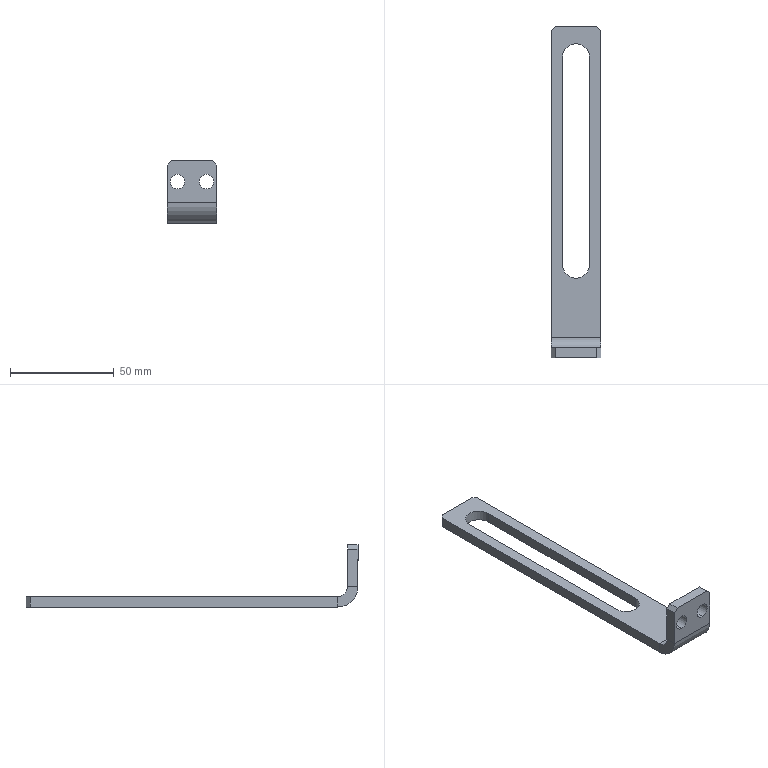Part | SolidWorks | 1 solid | 26 faces | box 24 x 160 x 30 mm | volume 14225 mm3 | plane 18 | cylinder 8 | commonest cylinder face diameters 7 x4 13 x2 10 x1 20 x1
STEP:
#1=CARTESIAN_POINT('',(-7.,-80.,18.5));
#2=VERTEX_POINT('',#1);
#3=CARTESIAN_POINT('',(-7.,-80.,11.5));
#4=VERTEX_POINT('',#3);
#5=CARTESIAN_POINT('',(-7.,-80.,15.));
#6=DIRECTION('',(0.,-1.,0.));
#7=DIRECTION('',(0.,0.,-1.));
#8=AXIS2_PLACEMENT_3D('',#5,#6,#7);
#9=CIRCLE('',#8,3.5);
#10=EDGE_CURVE('',#2,#4,#9,.T.);
#11=ORIENTED_EDGE('',*,*,#10,.T.);
#12=CARTESIAN_POINT('',(-7.,-75.,11.5));
#13=VERTEX_POINT('',#12);
#14=CARTESIAN_POINT('',(-7.,-85.,11.5));
#15=DIRECTION('',(0.,1.,0.));
#16=VECTOR('',#15,1000.);
#17=LINE('',#14,#16);
#18=EDGE_CURVE('',#4,#13,#17,.T.);
#19=ORIENTED_EDGE('',*,*,#18,.T.);
#20=CARTESIAN_POINT('',(-7.,-75.,18.5));
#21=VERTEX_POINT('',#20);
#22=CARTESIAN_POINT('',(-7.,-75.,15.));
#23=DIRECTION('',(0.,1.,0.));
#24=DIRECTION('',(0.,0.,1.));
#25=AXIS2_PLACEMENT_3D('',#22,#23,#24);
#26=CIRCLE('',#25,3.5);
#27=EDGE_CURVE('',#13,#21,#26,.T.);
#28=ORIENTED_EDGE('',*,*,#27,.T.);
#29=CARTESIAN_POINT('',(-7.,-85.,18.5));
#30=DIRECTION('',(0.,1.,0.));
#31=VECTOR('',#30,1000.);
#32=LINE('',#29,#31);
#33=EDGE_CURVE('',#2,#21,#32,.T.);
#34=ORIENTED_EDGE('',*,*,#33,.F.);
#35=EDGE_LOOP('',(#11,#19,#28,#34));
#36=FACE_OUTER_BOUND('',#35,.T.);
#37=CARTESIAN_POINT('',(-7.,-85.,15.));
#38=DIRECTION('',(0.,1.,0.));
#39=DIRECTION('',(0.,0.,1.));
#40=AXIS2_PLACEMENT_3D('',#37,#38,#39);
#41=CYLINDRICAL_SURFACE('',#40,3.5);
#42=ADVANCED_FACE('',(#36),#41,.F.);
#43=CARTESIAN_POINT('',(7.,-80.,18.5));
#44=VERTEX_POINT('',#43);
#45=CARTESIAN_POINT('',(7.,-80.,11.5));
#46=VERTEX_POINT('',#45);
#47=CARTESIAN_POINT('',(7.,-80.,15.));
#48=DIRECTION('',(0.,-1.,0.));
#49=DIRECTION('',(0.,0.,-1.));
#50=AXIS2_PLACEMENT_3D('',#47,#48,#49);
#51=CIRCLE('',#50,3.5);
#52=EDGE_CURVE('',#44,#46,#51,.T.);
#53=ORIENTED_EDGE('',*,*,#52,.T.);
#54=CARTESIAN_POINT('',(7.,-75.,11.5));
#55=VERTEX_POINT('',#54);
#56=CARTESIAN_POINT('',(7.,-85.,11.5));
#57=DIRECTION('',(0.,1.,0.));
#58=VECTOR('',#57,1000.);
#59=LINE('',#56,#58);
#60=EDGE_CURVE('',#46,#55,#59,.T.);
#61=ORIENTED_EDGE('',*,*,#60,.T.);
#62=CARTESIAN_POINT('',(7.,-75.,18.5));
#63=VERTEX_POINT('',#62);
#64=CARTESIAN_POINT('',(7.,-75.,15.));
#65=DIRECTION('',(0.,1.,0.));
#66=DIRECTION('',(0.,0.,1.));
#67=AXIS2_PLACEMENT_3D('',#64,#65,#66);
#68=CIRCLE('',#67,3.5);
#69=EDGE_CURVE('',#55,#63,#68,.T.);
#70=ORIENTED_EDGE('',*,*,#69,.T.);
#71=CARTESIAN_POINT('',(7.,-85.,18.5));
#72=DIRECTION('',(0.,1.,0.));
#73=VECTOR('',#72,1000.);
#74=LINE('',#71,#73);
#75=EDGE_CURVE('',#44,#63,#74,.T.);
#76=ORIENTED_EDGE('',*,*,#75,.F.);
#77=EDGE_LOOP('',(#53,#61,#70,#76));
#78=FACE_OUTER_BOUND('',#77,.T.);
#79=CARTESIAN_POINT('',(7.,-85.,15.));
#80=DIRECTION('',(0.,1.,0.));
#81=DIRECTION('',(0.,0.,1.));
#82=AXIS2_PLACEMENT_3D('',#79,#80,#81);
#83=CYLINDRICAL_SURFACE('',#82,3.5);
#84=ADVANCED_FACE('',(#78),#83,.F.);
#85=CARTESIAN_POINT('',(12.,-70.,-5.));
#86=VERTEX_POINT('',#85);
#87=CARTESIAN_POINT('',(12.,78.,-5.));
#88=VERTEX_POINT('',#87);
#89=CARTESIAN_POINT('',(12.,-80.,-5.));
#90=DIRECTION('',(0.,1.,0.));
#91=VECTOR('',#90,1000.);
#92=LINE('',#89,#91);
#93=EDGE_CURVE('',#86,#88,#92,.T.);
#94=ORIENTED_EDGE('',*,*,#93,.T.);
#95=CARTESIAN_POINT('',(12.,78.,0.));
#96=VERTEX_POINT('',#95);
#97=CARTESIAN_POINT('',(12.,78.,-5.));
#98=DIRECTION('',(0.,0.,1.));
#99=VECTOR('',#98,1000.);
#100=LINE('',#97,#99);
#101=EDGE_CURVE('',#88,#96,#100,.T.);
#102=ORIENTED_EDGE('',*,*,#101,.T.);
#103=CARTESIAN_POINT('',(12.,-70.,0.));
#104=VERTEX_POINT('',#103);
#105=CARTESIAN_POINT('',(12.,-80.,0.));
#106=DIRECTION('',(0.,1.,0.));
#107=VECTOR('',#106,1000.);
#108=LINE('',#105,#107);
#109=EDGE_CURVE('',#104,#96,#108,.T.);
#110=ORIENTED_EDGE('',*,*,#109,.F.);
#111=CARTESIAN_POINT('',(12.,-70.,0.));
#112=DIRECTION('',(0.,0.,-1.));
#113=VECTOR('',#112,1000.);
#114=LINE('',#111,#113);
#115=EDGE_CURVE('',#104,#86,#114,.T.);
#116=ORIENTED_EDGE('',*,*,#115,.T.);
#117=EDGE_LOOP('',(#94,#102,#110,#116));
#118=FACE_OUTER_BOUND('',#117,.T.);
#119=CARTESIAN_POINT('',(12.,-80.,-5.));
#120=DIRECTION('',(1.,0.,0.));
#121=DIRECTION('',(0.,0.,-1.));
#122=AXIS2_PLACEMENT_3D('',#119,#120,#121);
#123=PLANE('',#122);
#124=ADVANCED_FACE('',(#118),#123,.T.);
#125=CARTESIAN_POINT('',(-6.5,65.,-5.));
#126=VERTEX_POINT('',#125);
#127=CARTESIAN_POINT('',(6.5,65.,-5.));
#128=VERTEX_POINT('',#127);
#129=CARTESIAN_POINT('',(0.,65.,-5.));
#130=DIRECTION('',(0.,0.,-1.));
#131=DIRECTION('',(-1.,0.,0.));
#132=AXIS2_PLACEMENT_3D('',#129,#130,#131);
#133=CIRCLE('',#132,6.5);
#134=EDGE_CURVE('',#126,#128,#133,.T.);
#135=ORIENTED_EDGE('',*,*,#134,.F.);
#136=CARTESIAN_POINT('',(-6.5,-35.,-5.));
#137=VERTEX_POINT('',#136);
#138=CARTESIAN_POINT('',(-6.5,0.,-5.));
#139=DIRECTION('',(0.,1.,0.));
#140=VECTOR('',#139,1000.);
#141=LINE('',#138,#140);
#142=EDGE_CURVE('',#137,#126,#141,.T.);
#143=ORIENTED_EDGE('',*,*,#142,.F.);
#144=CARTESIAN_POINT('',(6.5,-35.,-5.));
#145=VERTEX_POINT('',#144);
#146=CARTESIAN_POINT('',(0.,-35.,-5.));
#147=DIRECTION('',(0.,0.,-1.));
#148=DIRECTION('',(-1.,0.,0.));
#149=AXIS2_PLACEMENT_3D('',#146,#147,#148);
#150=CIRCLE('',#149,6.5);
#151=EDGE_CURVE('',#145,#137,#150,.T.);
#152=ORIENTED_EDGE('',*,*,#151,.F.);
#153=CARTESIAN_POINT('',(6.5,0.,-5.));
#154=DIRECTION('',(0.,-1.,0.));
#155=VECTOR('',#154,1000.);
#156=LINE('',#153,#155);
#157=EDGE_CURVE('',#128,#145,#156,.T.);
#158=ORIENTED_EDGE('',*,*,#157,.F.);
#159=EDGE_LOOP('',(#135,#143,#152,#158));
#160=FACE_BOUND('',#159,.T.);
#161=CARTESIAN_POINT('',(10.,80.,-5.));
#162=VERTEX_POINT('',#161);
#163=CARTESIAN_POINT('',(-10.,80.,-5.));
#164=VERTEX_POINT('',#163);
#165=CARTESIAN_POINT('',(-12.,80.,-5.));
#166=DIRECTION('',(-1.,0.,0.));
#167=VECTOR('',#166,1000.);
#168=LINE('',#165,#167);
#169=EDGE_CURVE('',#162,#164,#168,.T.);
#170=ORIENTED_EDGE('',*,*,#169,.F.);
#171=CARTESIAN_POINT('',(45.,45.,-5.));
#172=DIRECTION('',(0.7071,-0.7071,0.));
#173=VECTOR('',#172,1000.);
#174=LINE('',#171,#173);
#175=EDGE_CURVE('',#162,#88,#174,.T.);
#176=ORIENTED_EDGE('',*,*,#175,.T.);
#177=ORIENTED_EDGE('',*,*,#93,.F.);
#178=CARTESIAN_POINT('',(-12.,-70.,-5.));
#179=VERTEX_POINT('',#178);
#180=CARTESIAN_POINT('',(12.,-70.,-5.));
#181=DIRECTION('',(-1.,0.,0.));
#182=VECTOR('',#181,1000.);
#183=LINE('',#180,#182);
#184=EDGE_CURVE('',#86,#179,#183,.T.);
#185=ORIENTED_EDGE('',*,*,#184,.T.);
#186=CARTESIAN_POINT('',(-12.,78.,-5.));
#187=VERTEX_POINT('',#186);
#188=CARTESIAN_POINT('',(-12.,-80.,-5.));
#189=DIRECTION('',(0.,-1.,0.));
#190=VECTOR('',#189,1000.);
#191=LINE('',#188,#190);
#192=EDGE_CURVE('',#187,#179,#191,.T.);
#193=ORIENTED_EDGE('',*,*,#192,.F.);
#194=CARTESIAN_POINT('',(-45.,45.,-5.));
#195=DIRECTION('',(0.7071,0.7071,0.));
#196=VECTOR('',#195,1000.);
#197=LINE('',#194,#196);
#198=EDGE_CURVE('',#187,#164,#197,.T.);
#199=ORIENTED_EDGE('',*,*,#198,.T.);
#200=EDGE_LOOP('',(#170,#176,#177,#185,#193,#199));
#201=FACE_OUTER_BOUND('',#200,.T.);
#202=CARTESIAN_POINT('',(0.,0.,-5.));
#203=DIRECTION('',(0.,0.,-1.));
#204=DIRECTION('',(-1.,0.,0.));
#205=AXIS2_PLACEMENT_3D('',#202,#203,#204);
#206=PLANE('',#205);
#207=ADVANCED_FACE('',(#160,#201),#206,.T.);
#208=CARTESIAN_POINT('',(-6.5,65.,0.));
#209=VERTEX_POINT('',#208);
#210=CARTESIAN_POINT('',(-6.5,-35.,0.));
#211=VERTEX_POINT('',#210);
#212=CARTESIAN_POINT('',(-6.5,65.,0.));
#213=DIRECTION('',(0.,-1.,0.));
#214=VECTOR('',#213,1000.);
#215=LINE('',#212,#214);
#216=EDGE_CURVE('',#209,#211,#215,.T.);
#217=ORIENTED_EDGE('',*,*,#216,.F.);
#218=CARTESIAN_POINT('',(6.5,65.,0.));
#219=VERTEX_POINT('',#218);
#220=CARTESIAN_POINT('',(0.,65.,0.));
#221=DIRECTION('',(0.,0.,1.));
#222=DIRECTION('',(1.,0.,0.));
#223=AXIS2_PLACEMENT_3D('',#220,#221,#222);
#224=CIRCLE('',#223,6.5);
#225=EDGE_CURVE('',#219,#209,#224,.T.);
#226=ORIENTED_EDGE('',*,*,#225,.F.);
#227=CARTESIAN_POINT('',(6.5,-35.,0.));
#228=VERTEX_POINT('',#227);
#229=CARTESIAN_POINT('',(6.5,65.,0.));
#230=DIRECTION('',(0.,1.,0.));
#231=VECTOR('',#230,1000.);
#232=LINE('',#229,#231);
#233=EDGE_CURVE('',#228,#219,#232,.T.);
#234=ORIENTED_EDGE('',*,*,#233,.F.);
#235=CARTESIAN_POINT('',(0.,-35.,0.));
#236=DIRECTION('',(0.,0.,1.));
#237=DIRECTION('',(1.,0.,0.));
#238=AXIS2_PLACEMENT_3D('',#235,#236,#237);
#239=CIRCLE('',#238,6.5);
#240=EDGE_CURVE('',#211,#228,#239,.T.);
#241=ORIENTED_EDGE('',*,*,#240,.F.);
#242=EDGE_LOOP('',(#217,#226,#234,#241));
#243=FACE_BOUND('',#242,.T.);
#244=ORIENTED_EDGE('',*,*,#109,.T.);
#245=CARTESIAN_POINT('',(10.,80.,0.));
#246=VERTEX_POINT('',#245);
#247=CARTESIAN_POINT('',(12.,78.,0.));
#248=DIRECTION('',(-0.7071,0.7071,0.));
#249=VECTOR('',#248,1000.);
#250=LINE('',#247,#249);
#251=EDGE_CURVE('',#96,#246,#250,.T.);
#252=ORIENTED_EDGE('',*,*,#251,.T.);
#253=CARTESIAN_POINT('',(-10.,80.,0.));
#254=VERTEX_POINT('',#253);
#255=CARTESIAN_POINT('',(-12.,80.,0.));
#256=DIRECTION('',(-1.,0.,0.));
#257=VECTOR('',#256,1000.);
#258=LINE('',#255,#257);
#259=EDGE_CURVE('',#246,#254,#258,.T.);
#260=ORIENTED_EDGE('',*,*,#259,.T.);
#261=CARTESIAN_POINT('',(-12.,78.,0.));
#262=VERTEX_POINT('',#261);
#263=CARTESIAN_POINT('',(-10.,80.,0.));
#264=DIRECTION('',(-0.7071,-0.7071,0.));
#265=VECTOR('',#264,1000.);
#266=LINE('',#263,#265);
#267=EDGE_CURVE('',#254,#262,#266,.T.);
#268=ORIENTED_EDGE('',*,*,#267,.T.);
#269=CARTESIAN_POINT('',(-12.,-70.,0.));
#270=VERTEX_POINT('',#269);
#271=CARTESIAN_POINT('',(-12.,-80.,0.));
#272=DIRECTION('',(0.,-1.,0.));
#273=VECTOR('',#272,1000.);
#274=LINE('',#271,#273);
#275=EDGE_CURVE('',#262,#270,#274,.T.);
#276=ORIENTED_EDGE('',*,*,#275,.T.);
#277=CARTESIAN_POINT('',(12.,-70.,0.));
#278=DIRECTION('',(-1.,0.,0.));
#279=VECTOR('',#278,1000.);
#280=LINE('',#277,#279);
#281=EDGE_CURVE('',#104,#270,#280,.T.);
#282=ORIENTED_EDGE('',*,*,#281,.F.);
#283=EDGE_LOOP('',(#244,#252,#260,#268,#276,#282));
#284=FACE_OUTER_BOUND('',#283,.T.);
#285=CARTESIAN_POINT('',(0.,0.,0.));
#286=DIRECTION('',(0.,0.,-1.));
#287=DIRECTION('',(-1.,0.,0.));
#288=AXIS2_PLACEMENT_3D('',#285,#286,#287);
#289=PLANE('',#288);
#290=ADVANCED_FACE('',(#243,#284),#289,.F.);
#291=ORIENTED_EDGE('',*,*,#275,.F.);
#292=CARTESIAN_POINT('',(-12.,78.,-5.));
#293=DIRECTION('',(0.,0.,-1.));
#294=VECTOR('',#293,1000.);
#295=LINE('',#292,#294);
#296=EDGE_CURVE('',#262,#187,#295,.T.);
#297=ORIENTED_EDGE('',*,*,#296,.T.);
#298=ORIENTED_EDGE('',*,*,#192,.T.);
#299=CARTESIAN_POINT('',(-12.,-70.,0.));
#300=DIRECTION('',(0.,0.,-1.));
#301=VECTOR('',#300,1000.);
#302=LINE('',#299,#301);
#303=EDGE_CURVE('',#270,#179,#302,.T.);
#304=ORIENTED_EDGE('',*,*,#303,.F.);
#305=EDGE_LOOP('',(#291,#297,#298,#304));
#306=FACE_OUTER_BOUND('',#305,.T.);
#307=CARTESIAN_POINT('',(-12.,-80.,-5.));
#308=DIRECTION('',(-1.,0.,0.));
#309=DIRECTION('',(0.,0.,1.));
#310=AXIS2_PLACEMENT_3D('',#307,#308,#309);
#311=PLANE('',#310);
#312=ADVANCED_FACE('',(#306),#311,.T.);
#313=ORIENTED_EDGE('',*,*,#259,.F.);
#314=CARTESIAN_POINT('',(10.,80.,-5.));
#315=DIRECTION('',(0.,0.,-1.));
#316=VECTOR('',#315,1000.);
#317=LINE('',#314,#316);
#318=EDGE_CURVE('',#246,#162,#317,.T.);
#319=ORIENTED_EDGE('',*,*,#318,.T.);
#320=ORIENTED_EDGE('',*,*,#169,.T.);
#321=CARTESIAN_POINT('',(-10.,80.,-5.));
#322=DIRECTION('',(0.,0.,1.));
#323=VECTOR('',#322,1000.);
#324=LINE('',#321,#323);
#325=EDGE_CURVE('',#164,#254,#324,.T.);
#326=ORIENTED_EDGE('',*,*,#325,.T.);
#327=EDGE_LOOP('',(#313,#319,#320,#326));
#328=FACE_OUTER_BOUND('',#327,.T.);
#329=CARTESIAN_POINT('',(-12.,80.,-5.));
#330=DIRECTION('',(0.,1.,0.));
#331=DIRECTION('',(0.,0.,1.));
#332=AXIS2_PLACEMENT_3D('',#329,#330,#331);
#333=PLANE('',#332);
#334=ADVANCED_FACE('',(#328),#333,.T.);
#335=CARTESIAN_POINT('',(-12.,-75.,5.));
#336=VERTEX_POINT('',#335);
#337=CARTESIAN_POINT('',(-12.,-80.,5.));
#338=VERTEX_POINT('',#337);
#339=CARTESIAN_POINT('',(-12.,-80.,5.));
#340=DIRECTION('',(0.,-1.,0.));
#341=VECTOR('',#340,1000.);
#342=LINE('',#339,#341);
#343=EDGE_CURVE('',#336,#338,#342,.T.);
#344=ORIENTED_EDGE('',*,*,#343,.F.);
#345=CARTESIAN_POINT('',(-12.,-70.,5.));
#346=DIRECTION('',(-1.,0.,0.));
#347=DIRECTION('',(0.,0.,-1.));
#348=AXIS2_PLACEMENT_3D('',#345,#346,#347);
#349=CIRCLE('',#348,5.);
#350=EDGE_CURVE('',#270,#336,#349,.T.);
#351=ORIENTED_EDGE('',*,*,#350,.F.);
#352=ORIENTED_EDGE('',*,*,#303,.T.);
#353=CARTESIAN_POINT('',(-12.,-70.,5.));
#354=DIRECTION('',(-1.,0.,0.));
#355=DIRECTION('',(0.,0.,-1.));
#356=AXIS2_PLACEMENT_3D('',#353,#354,#355);
#357=CIRCLE('',#356,10.);
#358=EDGE_CURVE('',#179,#338,#357,.T.);
#359=ORIENTED_EDGE('',*,*,#358,.T.);
#360=EDGE_LOOP('',(#344,#351,#352,#359));
#361=FACE_OUTER_BOUND('',#360,.T.);
#362=CARTESIAN_POINT('',(-12.,-70.,5.));
#363=DIRECTION('',(-1.,0.,0.));
#364=DIRECTION('',(0.,0.,1.));
#365=AXIS2_PLACEMENT_3D('',#362,#363,#364);
#366=PLANE('',#365);
#367=ADVANCED_FACE('',(#361),#366,.T.);
#368=CARTESIAN_POINT('',(12.,-75.,5.));
#369=VERTEX_POINT('',#368);
#370=CARTESIAN_POINT('',(12.,-70.,5.));
#371=DIRECTION('',(1.,0.,0.));
#372=DIRECTION('',(0.,0.,-1.));
#373=AXIS2_PLACEMENT_3D('',#370,#371,#372);
#374=CIRCLE('',#373,5.);
#375=EDGE_CURVE('',#369,#104,#374,.T.);
#376=ORIENTED_EDGE('',*,*,#375,.F.);
#377=CARTESIAN_POINT('',(12.,-80.,5.));
#378=VERTEX_POINT('',#377);
#379=CARTESIAN_POINT('',(12.,-75.,5.));
#380=DIRECTION('',(0.,-1.,0.));
#381=VECTOR('',#380,1000.);
#382=LINE('',#379,#381);
#383=EDGE_CURVE('',#369,#378,#382,.T.);
#384=ORIENTED_EDGE('',*,*,#383,.T.);
#385=CARTESIAN_POINT('',(12.,-70.,5.));
#386=DIRECTION('',(1.,0.,0.));
#387=DIRECTION('',(0.,0.,-1.));
#388=AXIS2_PLACEMENT_3D('',#385,#386,#387);
#389=CIRCLE('',#388,10.);
#390=EDGE_CURVE('',#378,#86,#389,.T.);
#391=ORIENTED_EDGE('',*,*,#390,.T.);
#392=ORIENTED_EDGE('',*,*,#115,.F.);
#393=EDGE_LOOP('',(#376,#384,#391,#392));
#394=FACE_OUTER_BOUND('',#393,.T.);
#395=CARTESIAN_POINT('',(12.,-70.,5.));
#396=DIRECTION('',(-1.,0.,0.));
#397=DIRECTION('',(0.,0.,1.));
#398=AXIS2_PLACEMENT_3D('',#395,#396,#397);
#399=PLANE('',#398);
#400=ADVANCED_FACE('',(#394),#399,.F.);
#401=ORIENTED_EDGE('',*,*,#184,.F.);
#402=ORIENTED_EDGE('',*,*,#390,.F.);
#403=CARTESIAN_POINT('',(0.,-80.,5.));
#404=DIRECTION('',(1.,0.,0.));
#405=VECTOR('',#404,1000.);
#406=LINE('',#403,#405);
#407=EDGE_CURVE('',#338,#378,#406,.T.);
#408=ORIENTED_EDGE('',*,*,#407,.F.);
#409=ORIENTED_EDGE('',*,*,#358,.F.);
#410=EDGE_LOOP('',(#401,#402,#408,#409));
#411=FACE_OUTER_BOUND('',#410,.T.);
#412=CARTESIAN_POINT('',(12.,-70.,5.));
#413=DIRECTION('',(1.,0.,0.));
#414=DIRECTION('',(0.,-1.,0.));
#415=AXIS2_PLACEMENT_3D('',#412,#413,#414);
#416=CYLINDRICAL_SURFACE('',#415,10.);
#417=ADVANCED_FACE('',(#411),#416,.T.);
#418=ORIENTED_EDGE('',*,*,#281,.T.);
#419=ORIENTED_EDGE('',*,*,#350,.T.);
#420=CARTESIAN_POINT('',(-12.,-75.,5.));
#421=DIRECTION('',(1.,0.,0.));
#422=VECTOR('',#421,1000.);
#423=LINE('',#420,#422);
#424=EDGE_CURVE('',#336,#369,#423,.T.);
#425=ORIENTED_EDGE('',*,*,#424,.T.);
#426=ORIENTED_EDGE('',*,*,#375,.T.);
#427=EDGE_LOOP('',(#418,#419,#425,#426));
#428=FACE_OUTER_BOUND('',#427,.T.);
#429=CARTESIAN_POINT('',(12.,-70.,5.));
#430=DIRECTION('',(1.,0.,0.));
#431=DIRECTION('',(0.,-1.,0.));
#432=AXIS2_PLACEMENT_3D('',#429,#430,#431);
#433=CYLINDRICAL_SURFACE('',#432,5.);
#434=ADVANCED_FACE('',(#428),#433,.F.);
#435=CARTESIAN_POINT('',(12.,-75.,23.));
#436=VERTEX_POINT('',#435);
#437=CARTESIAN_POINT('',(12.,-75.,0.));
#438=DIRECTION('',(0.,0.,-1.));
#439=VECTOR('',#438,1000.);
#440=LINE('',#437,#439);
#441=EDGE_CURVE('',#436,#369,#440,.T.);
#442=ORIENTED_EDGE('',*,*,#441,.F.);
#443=CARTESIAN_POINT('',(12.,-80.,23.));
#444=VERTEX_POINT('',#443);
#445=CARTESIAN_POINT('',(12.,-80.,23.));
#446=DIRECTION('',(0.,-1.,0.));
#447=VECTOR('',#446,1000.);
#448=LINE('',#445,#447);
#449=EDGE_CURVE('',#436,#444,#448,.T.);
#450=ORIENTED_EDGE('',*,*,#449,.T.);
#451=CARTESIAN_POINT('',(12.,-80.,0.));
#452=DIRECTION('',(0.,0.,-1.));
#453=VECTOR('',#452,1000.);
#454=LINE('',#451,#453);
#455=EDGE_CURVE('',#444,#378,#454,.T.);
#456=ORIENTED_EDGE('',*,*,#455,.T.);
#457=ORIENTED_EDGE('',*,*,#383,.F.);
#458=EDGE_LOOP('',(#442,#450,#456,#457));
#459=FACE_OUTER_BOUND('',#458,.T.);
#460=CARTESIAN_POINT('',(12.,-80.,0.));
#461=DIRECTION('',(1.,0.,0.));
#462=DIRECTION('',(0.,0.,-1.));
#463=AXIS2_PLACEMENT_3D('',#460,#461,#462);
#464=PLANE('',#463);
#465=ADVANCED_FACE('',(#459),#464,.T.);
#466=CARTESIAN_POINT('',(-12.,-80.,23.));
#467=VERTEX_POINT('',#466);
#468=CARTESIAN_POINT('',(-12.,-80.,25.));
#469=DIRECTION('',(0.,0.,1.));
#470=VECTOR('',#469,1000.);
#471=LINE('',#468,#470);
#472=EDGE_CURVE('',#338,#467,#471,.T.);
#473=ORIENTED_EDGE('',*,*,#472,.T.);
#474=CARTESIAN_POINT('',(-12.,-75.,23.));
#475=VERTEX_POINT('',#474);
#476=CARTESIAN_POINT('',(-12.,-80.,23.));
#477=DIRECTION('',(0.,1.,0.));
#478=VECTOR('',#477,1000.);
#479=LINE('',#476,#478);
#480=EDGE_CURVE('',#467,#475,#479,.T.);
#481=ORIENTED_EDGE('',*,*,#480,.T.);
#482=CARTESIAN_POINT('',(-12.,-75.,0.));
#483=DIRECTION('',(0.,0.,1.));
#484=VECTOR('',#483,1000.);
#485=LINE('',#482,#484);
#486=EDGE_CURVE('',#336,#475,#485,.T.);
#487=ORIENTED_EDGE('',*,*,#486,.F.);
#488=ORIENTED_EDGE('',*,*,#343,.T.);
#489=EDGE_LOOP('',(#473,#481,#487,#488));
#490=FACE_OUTER_BOUND('',#489,.T.);
#491=CARTESIAN_POINT('',(-12.,-80.,25.));
#492=DIRECTION('',(-1.,0.,0.));
#493=DIRECTION('',(0.,0.,1.));
#494=AXIS2_PLACEMENT_3D('',#491,#492,#493);
#495=PLANE('',#494);
#496=ADVANCED_FACE('',(#490),#495,.T.);
#497=ORIENTED_EDGE('',*,*,#10,.F.);
#498=CARTESIAN_POINT('',(-7.,-80.,15.));
#499=DIRECTION('',(0.,-1.,0.));
#500=DIRECTION('',(0.,0.,-1.));
#501=AXIS2_PLACEMENT_3D('',#498,#499,#500);
#502=CIRCLE('',#501,3.5);
#503=EDGE_CURVE('',#4,#2,#502,.T.);
#504=ORIENTED_EDGE('',*,*,#503,.F.);
#505=EDGE_LOOP('',(#497,#504));
#506=FACE_BOUND('',#505,.T.);
#507=ORIENTED_EDGE('',*,*,#52,.F.);
#508=CARTESIAN_POINT('',(7.,-80.,15.));
#509=DIRECTION('',(0.,-1.,0.));
#510=DIRECTION('',(0.,0.,-1.));
#511=AXIS2_PLACEMENT_3D('',#508,#509,#510);
#512=CIRCLE('',#511,3.5);
#513=EDGE_CURVE('',#46,#44,#512,.T.);
#514=ORIENTED_EDGE('',*,*,#513,.F.);
#515=EDGE_LOOP('',(#507,#514));
#516=FACE_BOUND('',#515,.T.);
#517=ORIENTED_EDGE('',*,*,#455,.F.);
#518=CARTESIAN_POINT('',(10.,-80.,25.));
#519=VERTEX_POINT('',#518);
#520=CARTESIAN_POINT('',(17.5,-80.,17.5));
#521=DIRECTION('',(-0.7071,0.,0.7071));
#522=VECTOR('',#521,1000.);
#523=LINE('',#520,#522);
#524=EDGE_CURVE('',#444,#519,#523,.T.);
#525=ORIENTED_EDGE('',*,*,#524,.T.);
#526=CARTESIAN_POINT('',(-10.,-80.,25.));
#527=VERTEX_POINT('',#526);
#528=CARTESIAN_POINT('',(12.,-80.,25.));
#529=DIRECTION('',(1.,0.,0.));
#530=VECTOR('',#529,1000.);
#531=LINE('',#528,#530);
#532=EDGE_CURVE('',#527,#519,#531,.T.);
#533=ORIENTED_EDGE('',*,*,#532,.F.);
#534=CARTESIAN_POINT('',(-17.5,-80.,17.5));
#535=DIRECTION('',(-0.7071,0.,-0.7071));
#536=VECTOR('',#535,1000.);
#537=LINE('',#534,#536);
#538=EDGE_CURVE('',#527,#467,#537,.T.);
#539=ORIENTED_EDGE('',*,*,#538,.T.);
#540=ORIENTED_EDGE('',*,*,#472,.F.);
#541=ORIENTED_EDGE('',*,*,#407,.T.);
#542=EDGE_LOOP('',(#517,#525,#533,#539,#540,#541));
#543=FACE_OUTER_BOUND('',#542,.T.);
#544=CARTESIAN_POINT('',(0.,-80.,0.));
#545=DIRECTION('',(0.,-1.,0.));
#546=DIRECTION('',(0.,0.,-1.));
#547=AXIS2_PLACEMENT_3D('',#544,#545,#546);
#548=PLANE('',#547);
#549=ADVANCED_FACE('',(#506,#516,#543),#548,.T.);
#550=CARTESIAN_POINT('',(-7.,-75.,15.));
#551=DIRECTION('',(0.,1.,0.));
#552=DIRECTION('',(0.,0.,1.));
#553=AXIS2_PLACEMENT_3D('',#550,#551,#552);
#554=CIRCLE('',#553,3.5);
#555=EDGE_CURVE('',#21,#13,#554,.T.);
#556=ORIENTED_EDGE('',*,*,#555,.F.);
#557=ORIENTED_EDGE('',*,*,#27,.F.);
#558=EDGE_LOOP('',(#556,#557));
#559=FACE_BOUND('',#558,.T.);
#560=CARTESIAN_POINT('',(7.,-75.,15.));
#561=DIRECTION('',(0.,1.,0.));
#562=DIRECTION('',(0.,0.,1.));
#563=AXIS2_PLACEMENT_3D('',#560,#561,#562);
#564=CIRCLE('',#563,3.5);
#565=EDGE_CURVE('',#63,#55,#564,.T.);
#566=ORIENTED_EDGE('',*,*,#565,.F.);
#567=ORIENTED_EDGE('',*,*,#69,.F.);
#568=EDGE_LOOP('',(#566,#567));
#569=FACE_BOUND('',#568,.T.);
#570=CARTESIAN_POINT('',(-10.,-75.,25.));
#571=VERTEX_POINT('',#570);
#572=CARTESIAN_POINT('',(10.,-75.,25.));
#573=VERTEX_POINT('',#572);
#574=CARTESIAN_POINT('',(0.,-75.,25.));
#575=DIRECTION('',(1.,0.,0.));
#576=VECTOR('',#575,1000.);
#577=LINE('',#574,#576);
#578=EDGE_CURVE('',#571,#573,#577,.T.);
#579=ORIENTED_EDGE('',*,*,#578,.T.);
#580=CARTESIAN_POINT('',(10.,-75.,25.));
#581=DIRECTION('',(0.7071,0.,-0.7071));
#582=VECTOR('',#581,1000.);
#583=LINE('',#580,#582);
#584=EDGE_CURVE('',#573,#436,#583,.T.);
#585=ORIENTED_EDGE('',*,*,#584,.T.);
#586=ORIENTED_EDGE('',*,*,#441,.T.);
#587=ORIENTED_EDGE('',*,*,#424,.F.);
#588=ORIENTED_EDGE('',*,*,#486,.T.);
#589=CARTESIAN_POINT('',(-12.,-75.,23.));
#590=DIRECTION('',(0.7071,0.,0.7071));
#591=VECTOR('',#590,1000.);
#592=LINE('',#589,#591);
#593=EDGE_CURVE('',#475,#571,#592,.T.);
#594=ORIENTED_EDGE('',*,*,#593,.T.);
#595=EDGE_LOOP('',(#579,#585,#586,#587,#588,#594));
#596=FACE_OUTER_BOUND('',#595,.T.);
#597=CARTESIAN_POINT('',(0.,-75.,0.));
#598=DIRECTION('',(0.,-1.,0.));
#599=DIRECTION('',(0.,0.,-1.));
#600=AXIS2_PLACEMENT_3D('',#597,#598,#599);
#601=PLANE('',#600);
#602=ADVANCED_FACE('',(#559,#569,#596),#601,.F.);
#603=ORIENTED_EDGE('',*,*,#532,.T.);
#604=CARTESIAN_POINT('',(10.,-80.,25.));
#605=DIRECTION('',(0.,1.,0.));
#606=VECTOR('',#605,1000.);
#607=LINE('',#604,#606);
#608=EDGE_CURVE('',#519,#573,#607,.T.);
#609=ORIENTED_EDGE('',*,*,#608,.T.);
#610=ORIENTED_EDGE('',*,*,#578,.F.);
#611=CARTESIAN_POINT('',(-10.,-80.,25.));
#612=DIRECTION('',(0.,-1.,0.));
#613=VECTOR('',#612,1000.);
#614=LINE('',#611,#613);
#615=EDGE_CURVE('',#571,#527,#614,.T.);
#616=ORIENTED_EDGE('',*,*,#615,.T.);
#617=EDGE_LOOP('',(#603,#609,#610,#616));
#618=FACE_OUTER_BOUND('',#617,.T.);
#619=CARTESIAN_POINT('',(12.,-80.,25.));
#620=DIRECTION('',(0.,0.,1.));
#621=DIRECTION('',(0.,-1.,0.));
#622=AXIS2_PLACEMENT_3D('',#619,#620,#621);
#623=PLANE('',#622);
#624=ADVANCED_FACE('',(#618),#623,.T.);
#625=ORIENTED_EDGE('',*,*,#175,.F.);
#626=ORIENTED_EDGE('',*,*,#318,.F.);
#627=ORIENTED_EDGE('',*,*,#251,.F.);
#628=ORIENTED_EDGE('',*,*,#101,.F.);
#629=EDGE_LOOP('',(#625,#626,#627,#628));
#630=FACE_OUTER_BOUND('',#629,.T.);
#631=CARTESIAN_POINT('',(12.,78.,-5.));
#632=DIRECTION('',(-0.7071,-0.7071,0.));
#633=DIRECTION('',(0.,0.,1.));
#634=AXIS2_PLACEMENT_3D('',#631,#632,#633);
#635=PLANE('',#634);
#636=ADVANCED_FACE('',(#630),#635,.F.);
#637=ORIENTED_EDGE('',*,*,#198,.F.);
#638=ORIENTED_EDGE('',*,*,#296,.F.);
#639=ORIENTED_EDGE('',*,*,#267,.F.);
#640=ORIENTED_EDGE('',*,*,#325,.F.);
#641=EDGE_LOOP('',(#637,#638,#639,#640));
#642=FACE_OUTER_BOUND('',#641,.T.);
#643=CARTESIAN_POINT('',(-10.,80.,-5.));
#644=DIRECTION('',(0.7071,-0.7071,0.));
#645=DIRECTION('',(0.,0.,1.));
#646=AXIS2_PLACEMENT_3D('',#643,#644,#645);
#647=PLANE('',#646);
#648=ADVANCED_FACE('',(#642),#647,.F.);
#649=ORIENTED_EDGE('',*,*,#524,.F.);
#650=ORIENTED_EDGE('',*,*,#449,.F.);
#651=ORIENTED_EDGE('',*,*,#584,.F.);
#652=ORIENTED_EDGE('',*,*,#608,.F.);
#653=EDGE_LOOP('',(#649,#650,#651,#652));
#654=FACE_OUTER_BOUND('',#653,.T.);
#655=CARTESIAN_POINT('',(10.,-80.,25.));
#656=DIRECTION('',(-0.7071,0.,-0.7071));
#657=DIRECTION('',(0.,1.,0.));
#658=AXIS2_PLACEMENT_3D('',#655,#656,#657);
#659=PLANE('',#658);
#660=ADVANCED_FACE('',(#654),#659,.F.);
#661=ORIENTED_EDGE('',*,*,#538,.F.);
#662=ORIENTED_EDGE('',*,*,#615,.F.);
#663=ORIENTED_EDGE('',*,*,#593,.F.);
#664=ORIENTED_EDGE('',*,*,#480,.F.);
#665=EDGE_LOOP('',(#661,#662,#663,#664));
#666=FACE_OUTER_BOUND('',#665,.T.);
#667=CARTESIAN_POINT('',(-12.,-80.,23.));
#668=DIRECTION('',(0.7071,0.,-0.7071));
#669=DIRECTION('',(0.,1.,0.));
#670=AXIS2_PLACEMENT_3D('',#667,#668,#669);
#671=PLANE('',#670);
#672=ADVANCED_FACE('',(#666),#671,.F.);
#673=ORIENTED_EDGE('',*,*,#134,.T.);
#674=CARTESIAN_POINT('',(6.5,65.,-10.));
#675=DIRECTION('',(0.,0.,1.));
#676=VECTOR('',#675,1000.);
#677=LINE('',#674,#676);
#678=EDGE_CURVE('',#128,#219,#677,.T.);
#679=ORIENTED_EDGE('',*,*,#678,.T.);
#680=ORIENTED_EDGE('',*,*,#225,.T.);
#681=CARTESIAN_POINT('',(-6.5,65.,-10.));
#682=DIRECTION('',(0.,0.,1.));
#683=VECTOR('',#682,1000.);
#684=LINE('',#681,#683);
#685=EDGE_CURVE('',#126,#209,#684,.T.);
#686=ORIENTED_EDGE('',*,*,#685,.F.);
#687=EDGE_LOOP('',(#673,#679,#680,#686));
#688=FACE_OUTER_BOUND('',#687,.T.);
#689=CARTESIAN_POINT('',(0.,65.,-10.));
#690=DIRECTION('',(0.,0.,1.));
#691=DIRECTION('',(1.,0.,0.));
#692=AXIS2_PLACEMENT_3D('',#689,#690,#691);
#693=CYLINDRICAL_SURFACE('',#692,6.5);
#694=ADVANCED_FACE('',(#688),#693,.F.);
#695=ORIENTED_EDGE('',*,*,#157,.T.);
#696=CARTESIAN_POINT('',(6.5,-35.,-10.));
#697=DIRECTION('',(0.,0.,1.));
#698=VECTOR('',#697,1000.);
#699=LINE('',#696,#698);
#700=EDGE_CURVE('',#145,#228,#699,.T.);
#701=ORIENTED_EDGE('',*,*,#700,.T.);
#702=ORIENTED_EDGE('',*,*,#233,.T.);
#703=ORIENTED_EDGE('',*,*,#678,.F.);
#704=EDGE_LOOP('',(#695,#701,#702,#703));
#705=FACE_OUTER_BOUND('',#704,.T.);
#706=CARTESIAN_POINT('',(6.5,65.,-10.));
#707=DIRECTION('',(1.,0.,0.));
#708=DIRECTION('',(0.,1.,0.));
#709=AXIS2_PLACEMENT_3D('',#706,#707,#708);
#710=PLANE('',#709);
#711=ADVANCED_FACE('',(#705),#710,.F.);
#712=ORIENTED_EDGE('',*,*,#151,.T.);
#713=CARTESIAN_POINT('',(-6.5,-35.,-10.));
#714=DIRECTION('',(0.,0.,1.));
#715=VECTOR('',#714,1000.);
#716=LINE('',#713,#715);
#717=EDGE_CURVE('',#137,#211,#716,.T.);
#718=ORIENTED_EDGE('',*,*,#717,.T.);
#719=ORIENTED_EDGE('',*,*,#240,.T.);
#720=ORIENTED_EDGE('',*,*,#700,.F.);
#721=EDGE_LOOP('',(#712,#718,#719,#720));
#722=FACE_OUTER_BOUND('',#721,.T.);
#723=CARTESIAN_POINT('',(0.,-35.,-10.));
#724=DIRECTION('',(0.,0.,1.));
#725=DIRECTION('',(1.,0.,0.));
#726=AXIS2_PLACEMENT_3D('',#723,#724,#725);
#727=CYLINDRICAL_SURFACE('',#726,6.5);
#728=ADVANCED_FACE('',(#722),#727,.F.);
#729=ORIENTED_EDGE('',*,*,#142,.T.);
#730=ORIENTED_EDGE('',*,*,#685,.T.);
#731=ORIENTED_EDGE('',*,*,#216,.T.);
#732=ORIENTED_EDGE('',*,*,#717,.F.);
#733=EDGE_LOOP('',(#729,#730,#731,#732));
#734=FACE_OUTER_BOUND('',#733,.T.);
#735=CARTESIAN_POINT('',(-6.5,65.,-10.));
#736=DIRECTION('',(-1.,0.,0.));
#737=DIRECTION('',(0.,-1.,0.));
#738=AXIS2_PLACEMENT_3D('',#735,#736,#737);
#739=PLANE('',#738);
#740=ADVANCED_FACE('',(#734),#739,.F.);
#741=ORIENTED_EDGE('',*,*,#60,.F.);
#742=ORIENTED_EDGE('',*,*,#513,.T.);
#743=ORIENTED_EDGE('',*,*,#75,.T.);
#744=ORIENTED_EDGE('',*,*,#565,.T.);
#745=EDGE_LOOP('',(#741,#742,#743,#744));
#746=FACE_OUTER_BOUND('',#745,.T.);
#747=CARTESIAN_POINT('',(7.,-85.,15.));
#748=DIRECTION('',(0.,1.,0.));
#749=DIRECTION('',(0.,0.,1.));
#750=AXIS2_PLACEMENT_3D('',#747,#748,#749);
#751=CYLINDRICAL_SURFACE('',#750,3.5);
#752=ADVANCED_FACE('',(#746),#751,.F.);
#753=ORIENTED_EDGE('',*,*,#18,.F.);
#754=ORIENTED_EDGE('',*,*,#503,.T.);
#755=ORIENTED_EDGE('',*,*,#33,.T.);
#756=ORIENTED_EDGE('',*,*,#555,.T.);
#757=EDGE_LOOP('',(#753,#754,#755,#756));
#758=FACE_OUTER_BOUND('',#757,.T.);
#759=CARTESIAN_POINT('',(-7.,-85.,15.));
#760=DIRECTION('',(0.,1.,0.));
#761=DIRECTION('',(0.,0.,1.));
#762=AXIS2_PLACEMENT_3D('',#759,#760,#761);
#763=CYLINDRICAL_SURFACE('',#762,3.5);
#764=ADVANCED_FACE('',(#758),#763,.F.);
#765=CLOSED_SHELL('',(#42,#84,#124,#207,#290,#312,#334,#367,#400,#417,#434,#465,#496,#549,#602,#624,#636,#648,#660,#672,#694,#711,#728,#740,#752,#764));
#766=MANIFOLD_SOLID_BREP('',#765);
#767=CARTESIAN_POINT('',(0.,0.,0.));
#768=DIRECTION('',(0.,0.,1.));
#769=DIRECTION('',(1.,0.,0.));
#770=AXIS2_PLACEMENT_3D('',#767,#768,#769);
#771=(LENGTH_UNIT()NAMED_UNIT(*)SI_UNIT(.MILLI.,.METRE.));
#772=UNCERTAINTY_MEASURE_WITH_UNIT(LENGTH_MEASURE(0.00001),#771,'','');
#773=(NAMED_UNIT(*)PLANE_ANGLE_UNIT()SI_UNIT($,.RADIAN.));
#774=(NAMED_UNIT(*)SI_UNIT($,.STERADIAN.)SOLID_ANGLE_UNIT());
#775=(GEOMETRIC_REPRESENTATION_CONTEXT(3)GLOBAL_UNCERTAINTY_ASSIGNED_CONTEXT((#772))GLOBAL_UNIT_ASSIGNED_CONTEXT((#771,#773,#774))REPRESENTATION_CONTEXT('',''));
#776=ADVANCED_BREP_SHAPE_REPRESENTATION('',(#766,#770),#775);